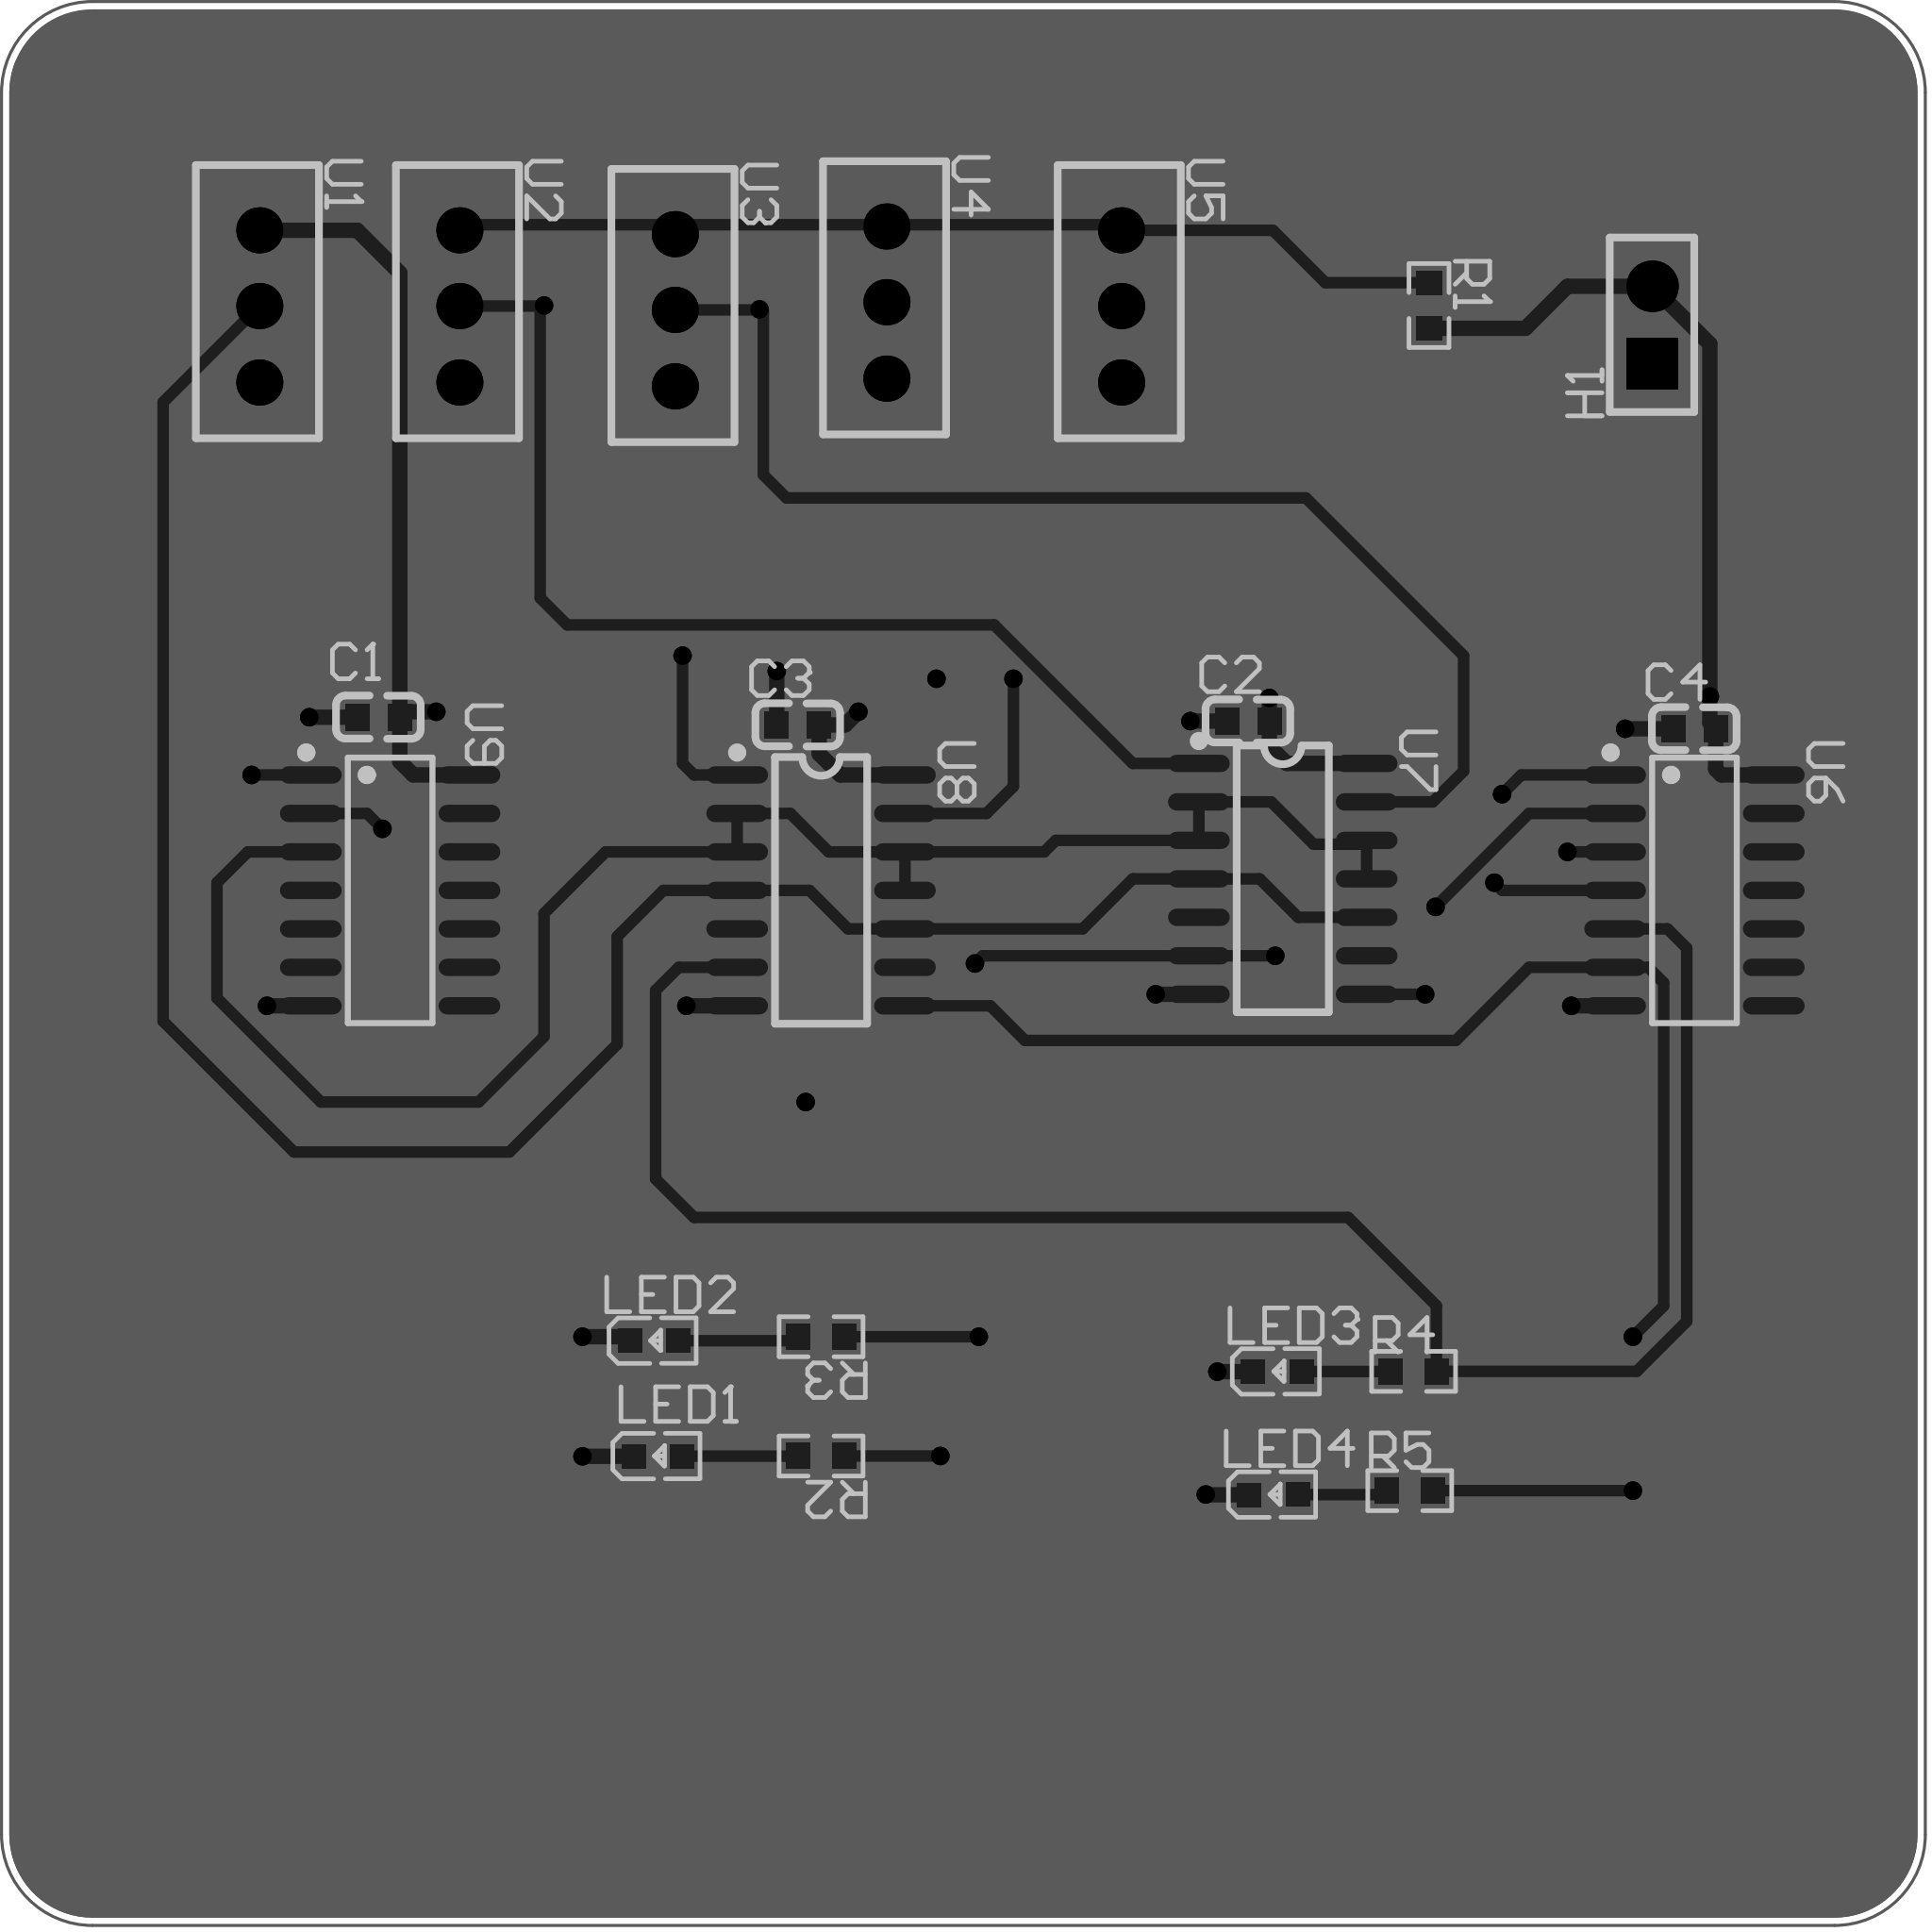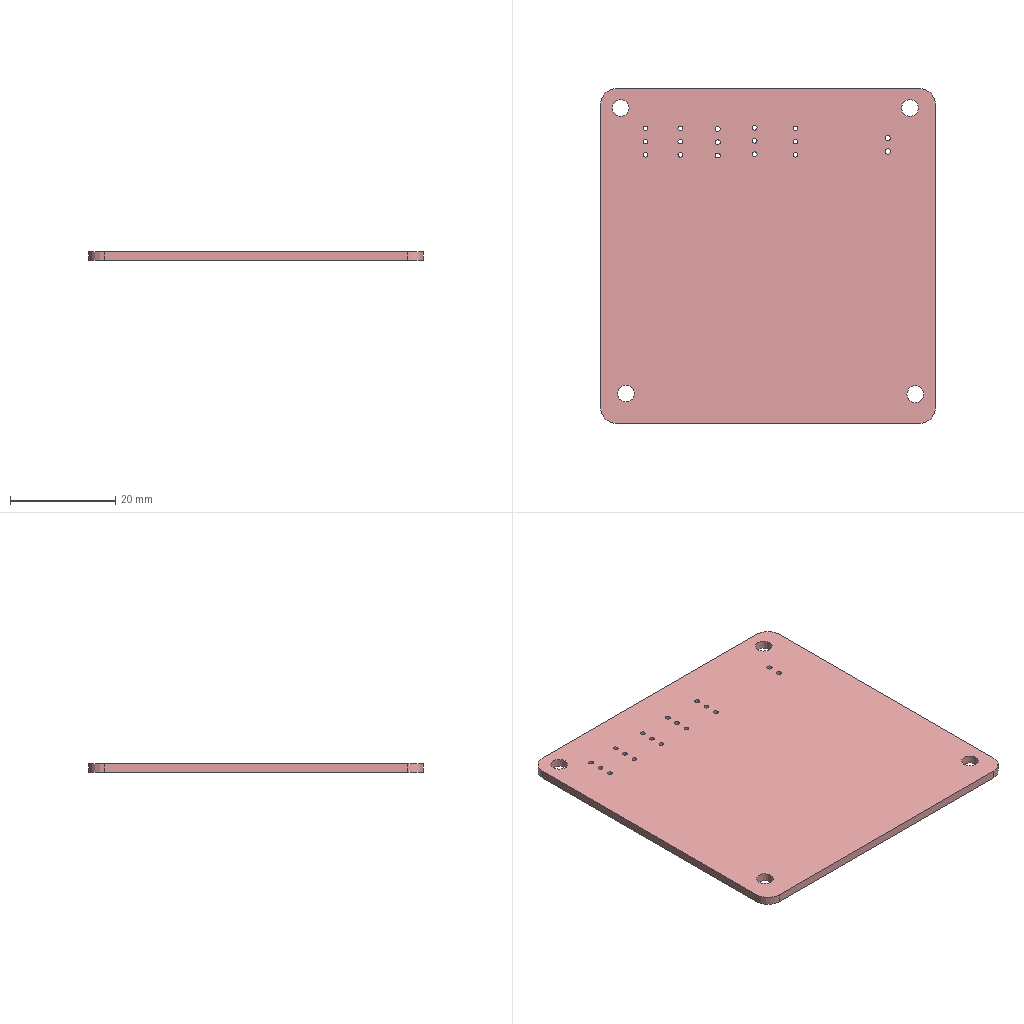Circuit board layout | Altium Designer | box 63.5 x 63.5 x 1.6 mm
Layer stack:
# Altium Designer layer stack of  (unit mm; dielectric type: 0 none, 1 core, 2 prepreg, 3 surface material)
index,name,kind,layer,copper_thickness_mm,dielectric_type,dielectric_thickness_mm,dielectric_material,dielectric_constant
0,Top Paste Mask Layer,other,,,,,,
1,Top Silkscreen Layer,other,,,,,,
2,Top Solder Mask Layer,dielectric,,,3,0.01,,3.3
3,Top Layer,copper,Top Layer,0.035,,,,
4,Dielectric1,dielectric,,,3,1.51,FR4,4.5
5,Bottom Layer,copper,Bottom Layer,0.035,,,,
6,Bottom Solder Mask Layer,dielectric,,,3,0.01,,3.3
7,Bottom Silkscreen Layer,other,,,,,,
8,Bottom Paste Mask Layer,other,,,,,,
# drill layer pairs: low layer,high layer
drill_pair,Top Layer,Bottom Layer
Part placement:
Designator,Comment,Layer,Footprint,Center-X(mm),Center-Y(mm),Rotation
C1,100nF,TopLayer,C0603,94.107,132.461,0
C2,100nF,TopLayer,C0603,122.809,132.334,0
C3,100nF,TopLayer,C0603,107.95,132.207,0
C4,100nF,TopLayer,C0603,137.541,132.08,0
H1,,TopLayer,HDR-TH_2P-P2.54-V-F,136.144,145.415,90
LED1,,TopLayer,LED_0603,103.327,108.069,0
LED2,,TopLayer,LED_0603,103.2,111.879,0
LED3,,TopLayer,LED_0603,123.774,110.863,0
LED4,,TopLayer,LED_0603,123.647,106.799,0
R1,0.1k,TopLayer,R0603,128.778,146.05,270
R2,10K,TopLayer,R0603,108.712,108.077,180
R3,10K,TopLayer,R0603,108.712,112.014,180
R4,10K,TopLayer,R0603,128.27,110.871,180
R5,10K,TopLayer,R0603,128.143,106.934,180
U1,,TopLayer,单刀双掷,90.17,146.021,270
U2,,TopLayer,单刀双掷,96.774,146.021,270
U3,,TopLayer,单刀双掷,103.886,145.894,270
U4,,TopLayer,单刀双掷,110.871,146.148,270
U5,,TopLayer,单刀双掷,118.618,146.021,270
U6,SN74LS02DRE4,TopLayer,SOIC-14_L8.7-W3.9-P1.27-LS6.0-BL,137.541,126.746,270
U7,SN74LS113ADR,TopLayer,SOIC-14_L8.6-W3.9-P1.27-LS6.0-BL,123.952,127.127,270
U8,SN74LS113ADR,TopLayer,SOIC-14_L8.6-W3.9-P1.27-LS6.0-BL,108.712,126.746,270
U9,SN74LS08DTR(XBLW),TopLayer,SOIC-14_L8.7-W3.9-P1.27-LS6.0-BL,94.488,126.746,270
Pad and via stacks:
# Altium Designer via and pad stacks of  (unit mm). Each distinct definition once, with the count of objects using it.
# via: kind,start_layer,end_layer,hole_mm,diameter_mm,mode(0 simple;1 top-mid-bottom;2 full stack),diameter_per_layer,count,example_net
# pad: kind,layer,hole_mm,hole_type(0 round;1 square;2 slot),plating,top_size,top_shape(1 round;2 rect;3 octagon;9 rounded rect),mid_size,bottom_size,mode,footprint,size_per_layer,count,example
pad,Top Layer,0,0,plated,0.8x0.9,2,0.8x0.9,0.8x0.9,0,C0603,,8,C1.2
pad,Top Layer,0,0,plated,0.8001x0.8001,2,0.8001x0.8001,0.8001x0.8001,0,LED_0603,,8,LED1.1
pad,Top Layer,0,0,plated,0.8065x0.864,2,0.8065x0.864,0.8065x0.864,0,R0603,,10,R1.2
pad,Top Layer,0,0,plated,0.574x2.038,1,0.574x2.038,0.574x2.038,0,SOIC-14_L8.7-W3.9-P1.27-LS6.0-BL,,28,U6.8
pad,Top Layer,0,0,plated,0.574x2.038,1,0.574x2.038,0.574x2.038,0,SOIC-14_L8.6-W3.9-P1.27-LS6.0-BL,,28,U7.8
pad,Multi-Layer,1,0,plated,1.7x1.7,2,1.7x1.7,1.7x1.7,0,HDR-TH_2P-P2.54-V-F,,1,H1.1
pad,Multi-Layer,1,0,plated,1.7x1.7,1,1.7x1.7,1.7x1.7,0,HDR-TH_2P-P2.54-V-F,,1,H1.2
pad,Multi-Layer,0.9144,0,plated,1.524x1.524,1,1.524x1.524,1.524x1.524,0,\u00B5\u00A5\u00B5\u00B6\u00CB\u00AB\u00D6\u00C0,,15,U1.1
via,Top Layer,Bottom Layer,0.3048,0.61,0,,35,$1N18
Copper pours:
name,layer,net,type(0 solid;1 hatched;2 none)
Bottom Layer-GND,Bottom Layer,GND,0
Bottom Layer-GND 1,Bottom Layer,GND,0
Design rules, without the lines most boards share:
# Altium Designer design rules of  (exported by Altium Designer, unit mm)
# columns: name | kind | enabled | priority | scope1 | scope2 | descriptor | typed fields (field=value)
pwr | 2 | enabled | 2 | (InNet('GND') OR InNet('VCC')) | All | Width Constraint (Min=5mil) (Max=100mil) (Preferred=20mil) ((InNet('GND') OR InNet('VCC'))) |
copperThickness1oz_2 | 2 | enabled | 3 | All | All | Width Constraint (Min=5mil) (Max=100mil) (Preferred=15mil) (All) |